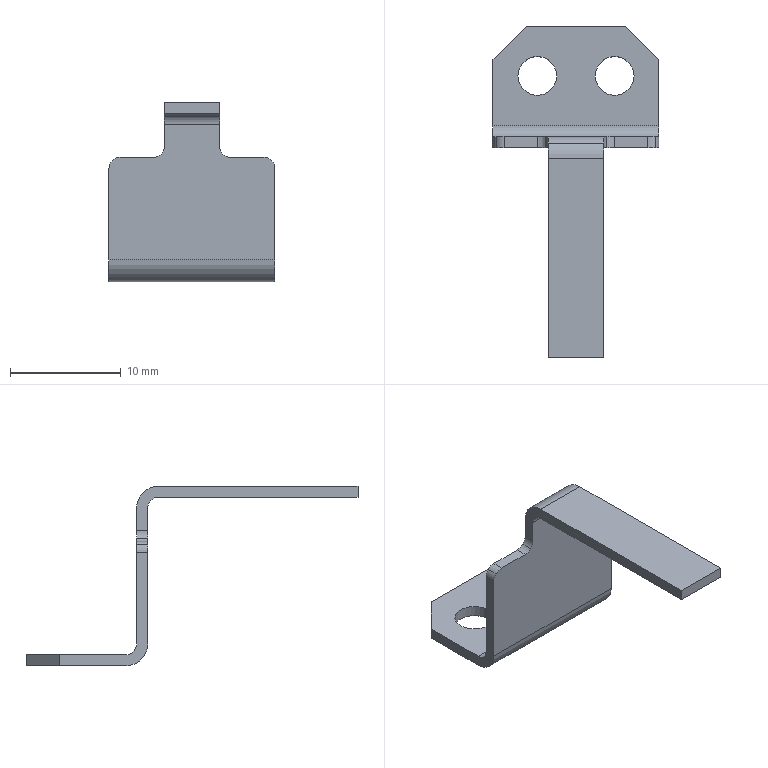Part | STEP file | ASND-0110-DH2TC90-28(2) | 1 solid | 34 faces | box 15 x 30 x 16.25 mm | volume 397.632 mm3 | cylinder 18 | plane 16 | commonest cylinder face diameters 2 x11 3.5 x4 4 x3